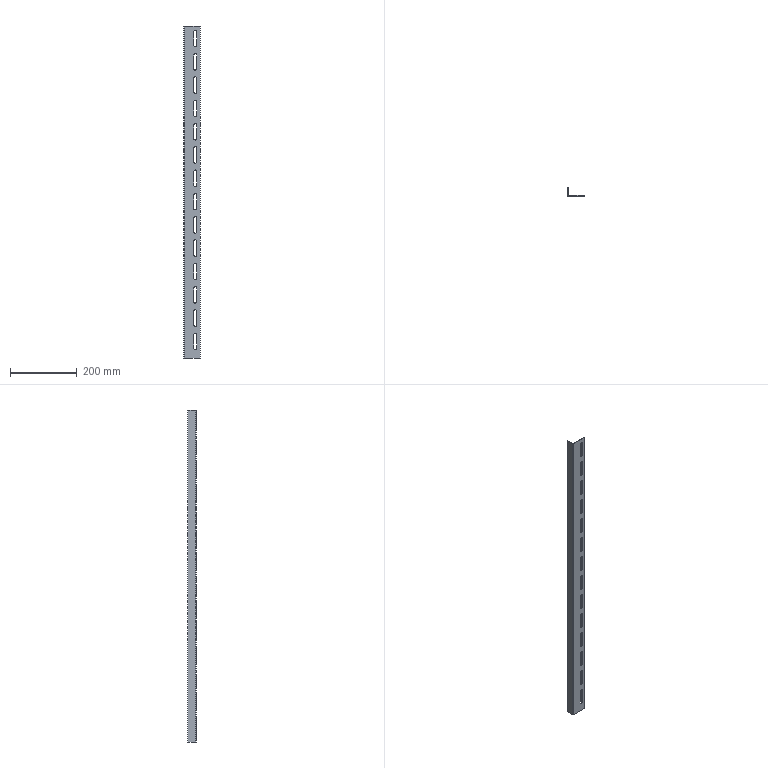Part | SolidWorks | features BaseBody 1 | 1 solid | 80 faces | box 50 x 25 x 997.6 mm | volume 119077 mm3 | cylinder 44 | plane 36 | commonest cylinder face diameters 9 x42 2 x1 5.6 x1